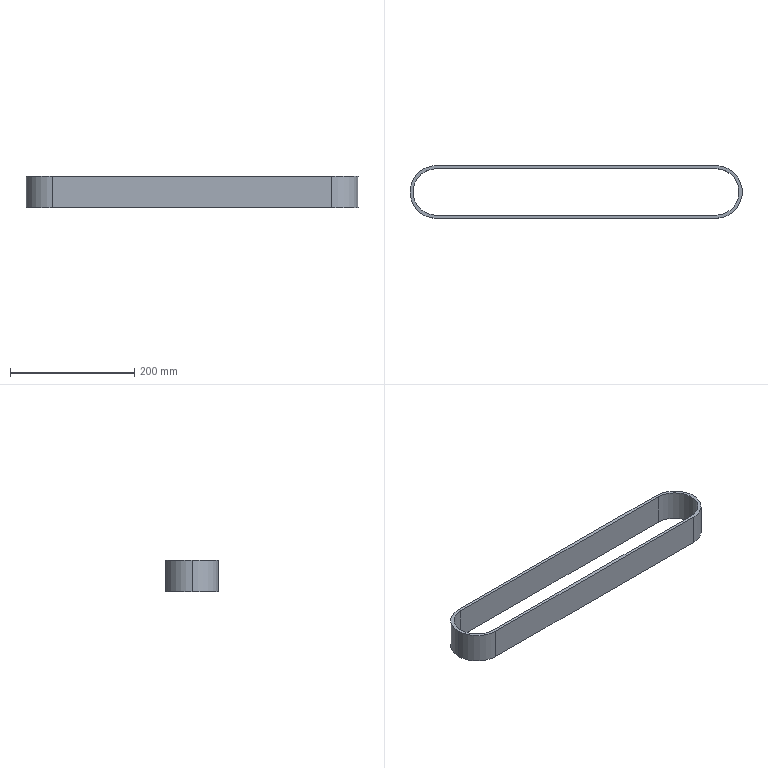Part | SolidWorks | features Extrusion 1 | 1 solid | 12 faces | box 535 x 85 x 50 mm | volume 287832 mm3 | cylinder 6 | plane 6 | commonest cylinder face diameters 75 x3 85 x3
STEP:
#1=CARTESIAN_POINT('',(-225.,37.5,50.));
#2=VERTEX_POINT('',#1);
#3=CARTESIAN_POINT('',(-262.5,0.,50.));
#4=VERTEX_POINT('',#3);
#5=CARTESIAN_POINT('',(-225.,0.,50.));
#6=DIRECTION('',(0.,0.,1.));
#7=DIRECTION('',(1.,0.,0.));
#8=AXIS2_PLACEMENT_3D('',#5,#6,#7);
#9=CIRCLE('',#8,37.5);
#10=EDGE_CURVE('',#2,#4,#9,.T.);
#11=ORIENTED_EDGE('',*,*,#10,.T.);
#12=CARTESIAN_POINT('',(-262.5,0.,0.));
#13=VERTEX_POINT('',#12);
#14=CARTESIAN_POINT('',(-262.5,0.,50.));
#15=DIRECTION('',(0.,0.,-1.));
#16=VECTOR('',#15,1000.);
#17=LINE('',#14,#16);
#18=EDGE_CURVE('',#4,#13,#17,.T.);
#19=ORIENTED_EDGE('',*,*,#18,.T.);
#20=CARTESIAN_POINT('',(-225.,37.5,0.));
#21=VERTEX_POINT('',#20);
#22=CARTESIAN_POINT('',(-225.,0.,0.));
#23=DIRECTION('',(0.,0.,1.));
#24=DIRECTION('',(1.,0.,0.));
#25=AXIS2_PLACEMENT_3D('',#22,#23,#24);
#26=CIRCLE('',#25,37.5);
#27=EDGE_CURVE('',#21,#13,#26,.T.);
#28=ORIENTED_EDGE('',*,*,#27,.F.);
#29=CARTESIAN_POINT('',(-225.,37.5,50.));
#30=DIRECTION('',(0.,0.,-1.));
#31=VECTOR('',#30,1000.);
#32=LINE('',#29,#31);
#33=EDGE_CURVE('',#2,#21,#32,.T.);
#34=ORIENTED_EDGE('',*,*,#33,.F.);
#35=EDGE_LOOP('',(#11,#19,#28,#34));
#36=FACE_OUTER_BOUND('',#35,.T.);
#37=CARTESIAN_POINT('',(-225.,0.,50.));
#38=DIRECTION('',(0.,0.,-1.));
#39=DIRECTION('',(-1.,0.,0.));
#40=AXIS2_PLACEMENT_3D('',#37,#38,#39);
#41=CYLINDRICAL_SURFACE('',#40,37.5);
#42=ADVANCED_FACE('',(#36),#41,.F.);
#43=CARTESIAN_POINT('',(-267.5,0.,50.));
#44=VERTEX_POINT('',#43);
#45=CARTESIAN_POINT('',(-225.,-42.5,50.));
#46=VERTEX_POINT('',#45);
#47=CARTESIAN_POINT('',(-225.,0.,50.));
#48=DIRECTION('',(0.,0.,1.));
#49=DIRECTION('',(1.,0.,0.));
#50=AXIS2_PLACEMENT_3D('',#47,#48,#49);
#51=CIRCLE('',#50,42.5);
#52=EDGE_CURVE('',#44,#46,#51,.T.);
#53=ORIENTED_EDGE('',*,*,#52,.F.);
#54=CARTESIAN_POINT('',(-267.5,0.,0.));
#55=VERTEX_POINT('',#54);
#56=CARTESIAN_POINT('',(-267.5,0.,50.));
#57=DIRECTION('',(0.,0.,-1.));
#58=VECTOR('',#57,1000.);
#59=LINE('',#56,#58);
#60=EDGE_CURVE('',#44,#55,#59,.T.);
#61=ORIENTED_EDGE('',*,*,#60,.T.);
#62=CARTESIAN_POINT('',(-225.,-42.5,0.));
#63=VERTEX_POINT('',#62);
#64=CARTESIAN_POINT('',(-225.,0.,0.));
#65=DIRECTION('',(0.,0.,1.));
#66=DIRECTION('',(1.,0.,0.));
#67=AXIS2_PLACEMENT_3D('',#64,#65,#66);
#68=CIRCLE('',#67,42.5);
#69=EDGE_CURVE('',#55,#63,#68,.T.);
#70=ORIENTED_EDGE('',*,*,#69,.T.);
#71=CARTESIAN_POINT('',(-225.,-42.5,50.));
#72=DIRECTION('',(0.,0.,-1.));
#73=VECTOR('',#72,1000.);
#74=LINE('',#71,#73);
#75=EDGE_CURVE('',#46,#63,#74,.T.);
#76=ORIENTED_EDGE('',*,*,#75,.F.);
#77=EDGE_LOOP('',(#53,#61,#70,#76));
#78=FACE_OUTER_BOUND('',#77,.T.);
#79=CARTESIAN_POINT('',(-225.,0.,50.));
#80=DIRECTION('',(0.,0.,-1.));
#81=DIRECTION('',(-1.,0.,0.));
#82=AXIS2_PLACEMENT_3D('',#79,#80,#81);
#83=CYLINDRICAL_SURFACE('',#82,42.5);
#84=ADVANCED_FACE('',(#78),#83,.T.);
#85=CARTESIAN_POINT('',(-225.,42.5,50.));
#86=VERTEX_POINT('',#85);
#87=CARTESIAN_POINT('',(-225.,0.,50.));
#88=DIRECTION('',(0.,0.,1.));
#89=DIRECTION('',(1.,0.,0.));
#90=AXIS2_PLACEMENT_3D('',#87,#88,#89);
#91=CIRCLE('',#90,42.5);
#92=EDGE_CURVE('',#86,#44,#91,.T.);
#93=ORIENTED_EDGE('',*,*,#92,.T.);
#94=ORIENTED_EDGE('',*,*,#52,.T.);
#95=CARTESIAN_POINT('',(225.,-42.5,50.));
#96=VERTEX_POINT('',#95);
#97=CARTESIAN_POINT('',(-225.,-42.5,50.));
#98=DIRECTION('',(1.,0.,0.));
#99=VECTOR('',#98,1000.);
#100=LINE('',#97,#99);
#101=EDGE_CURVE('',#46,#96,#100,.T.);
#102=ORIENTED_EDGE('',*,*,#101,.T.);
#103=CARTESIAN_POINT('',(225.,42.5,50.));
#104=VERTEX_POINT('',#103);
#105=CARTESIAN_POINT('',(225.,0.,50.));
#106=DIRECTION('',(0.,0.,1.));
#107=DIRECTION('',(1.,0.,0.));
#108=AXIS2_PLACEMENT_3D('',#105,#106,#107);
#109=CIRCLE('',#108,42.5);
#110=EDGE_CURVE('',#96,#104,#109,.T.);
#111=ORIENTED_EDGE('',*,*,#110,.T.);
#112=CARTESIAN_POINT('',(-225.,42.5,50.));
#113=DIRECTION('',(-1.,0.,0.));
#114=VECTOR('',#113,1000.);
#115=LINE('',#112,#114);
#116=EDGE_CURVE('',#104,#86,#115,.T.);
#117=ORIENTED_EDGE('',*,*,#116,.T.);
#118=EDGE_LOOP('',(#93,#94,#102,#111,#117));
#119=FACE_OUTER_BOUND('',#118,.T.);
#120=CARTESIAN_POINT('',(-225.,-37.5,50.));
#121=VERTEX_POINT('',#120);
#122=CARTESIAN_POINT('',(225.,-37.5,50.));
#123=VERTEX_POINT('',#122);
#124=CARTESIAN_POINT('',(-225.,-37.5,50.));
#125=DIRECTION('',(1.,0.,0.));
#126=VECTOR('',#125,1000.);
#127=LINE('',#124,#126);
#128=EDGE_CURVE('',#121,#123,#127,.T.);
#129=ORIENTED_EDGE('',*,*,#128,.F.);
#130=CARTESIAN_POINT('',(-225.,0.,50.));
#131=DIRECTION('',(0.,0.,1.));
#132=DIRECTION('',(1.,0.,0.));
#133=AXIS2_PLACEMENT_3D('',#130,#131,#132);
#134=CIRCLE('',#133,37.5);
#135=EDGE_CURVE('',#4,#121,#134,.T.);
#136=ORIENTED_EDGE('',*,*,#135,.F.);
#137=ORIENTED_EDGE('',*,*,#10,.F.);
#138=CARTESIAN_POINT('',(225.,37.5,50.));
#139=VERTEX_POINT('',#138);
#140=CARTESIAN_POINT('',(-225.,37.5,50.));
#141=DIRECTION('',(-1.,0.,0.));
#142=VECTOR('',#141,1000.);
#143=LINE('',#140,#142);
#144=EDGE_CURVE('',#139,#2,#143,.T.);
#145=ORIENTED_EDGE('',*,*,#144,.F.);
#146=CARTESIAN_POINT('',(225.,0.,50.));
#147=DIRECTION('',(0.,0.,1.));
#148=DIRECTION('',(1.,0.,0.));
#149=AXIS2_PLACEMENT_3D('',#146,#147,#148);
#150=CIRCLE('',#149,37.5);
#151=EDGE_CURVE('',#123,#139,#150,.T.);
#152=ORIENTED_EDGE('',*,*,#151,.F.);
#153=EDGE_LOOP('',(#129,#136,#137,#145,#152));
#154=FACE_BOUND('',#153,.T.);
#155=CARTESIAN_POINT('',(-225.,0.,50.));
#156=DIRECTION('',(0.,0.,1.));
#157=DIRECTION('',(1.,0.,0.));
#158=AXIS2_PLACEMENT_3D('',#155,#156,#157);
#159=PLANE('',#158);
#160=ADVANCED_FACE('',(#119,#154),#159,.T.);
#161=CARTESIAN_POINT('',(-225.,42.5,0.));
#162=VERTEX_POINT('',#161);
#163=CARTESIAN_POINT('',(-225.,0.,0.));
#164=DIRECTION('',(0.,0.,1.));
#165=DIRECTION('',(1.,0.,0.));
#166=AXIS2_PLACEMENT_3D('',#163,#164,#165);
#167=CIRCLE('',#166,42.5);
#168=EDGE_CURVE('',#162,#55,#167,.T.);
#169=ORIENTED_EDGE('',*,*,#168,.F.);
#170=CARTESIAN_POINT('',(225.,42.5,0.));
#171=VERTEX_POINT('',#170);
#172=CARTESIAN_POINT('',(-225.,42.5,0.));
#173=DIRECTION('',(-1.,0.,0.));
#174=VECTOR('',#173,1000.);
#175=LINE('',#172,#174);
#176=EDGE_CURVE('',#171,#162,#175,.T.);
#177=ORIENTED_EDGE('',*,*,#176,.F.);
#178=CARTESIAN_POINT('',(225.,-42.5,0.));
#179=VERTEX_POINT('',#178);
#180=CARTESIAN_POINT('',(225.,0.,0.));
#181=DIRECTION('',(0.,0.,1.));
#182=DIRECTION('',(1.,0.,0.));
#183=AXIS2_PLACEMENT_3D('',#180,#181,#182);
#184=CIRCLE('',#183,42.5);
#185=EDGE_CURVE('',#179,#171,#184,.T.);
#186=ORIENTED_EDGE('',*,*,#185,.F.);
#187=CARTESIAN_POINT('',(-225.,-42.5,0.));
#188=DIRECTION('',(1.,0.,0.));
#189=VECTOR('',#188,1000.);
#190=LINE('',#187,#189);
#191=EDGE_CURVE('',#63,#179,#190,.T.);
#192=ORIENTED_EDGE('',*,*,#191,.F.);
#193=ORIENTED_EDGE('',*,*,#69,.F.);
#194=EDGE_LOOP('',(#169,#177,#186,#192,#193));
#195=FACE_OUTER_BOUND('',#194,.T.);
#196=ORIENTED_EDGE('',*,*,#27,.T.);
#197=CARTESIAN_POINT('',(-225.,-37.5,0.));
#198=VERTEX_POINT('',#197);
#199=CARTESIAN_POINT('',(-225.,0.,0.));
#200=DIRECTION('',(0.,0.,1.));
#201=DIRECTION('',(1.,0.,0.));
#202=AXIS2_PLACEMENT_3D('',#199,#200,#201);
#203=CIRCLE('',#202,37.5);
#204=EDGE_CURVE('',#13,#198,#203,.T.);
#205=ORIENTED_EDGE('',*,*,#204,.T.);
#206=CARTESIAN_POINT('',(225.,-37.5,0.));
#207=VERTEX_POINT('',#206);
#208=CARTESIAN_POINT('',(-225.,-37.5,0.));
#209=DIRECTION('',(1.,0.,0.));
#210=VECTOR('',#209,1000.);
#211=LINE('',#208,#210);
#212=EDGE_CURVE('',#198,#207,#211,.T.);
#213=ORIENTED_EDGE('',*,*,#212,.T.);
#214=CARTESIAN_POINT('',(225.,37.5,0.));
#215=VERTEX_POINT('',#214);
#216=CARTESIAN_POINT('',(225.,0.,0.));
#217=DIRECTION('',(0.,0.,1.));
#218=DIRECTION('',(1.,0.,0.));
#219=AXIS2_PLACEMENT_3D('',#216,#217,#218);
#220=CIRCLE('',#219,37.5);
#221=EDGE_CURVE('',#207,#215,#220,.T.);
#222=ORIENTED_EDGE('',*,*,#221,.T.);
#223=CARTESIAN_POINT('',(-225.,37.5,0.));
#224=DIRECTION('',(-1.,0.,0.));
#225=VECTOR('',#224,1000.);
#226=LINE('',#223,#225);
#227=EDGE_CURVE('',#215,#21,#226,.T.);
#228=ORIENTED_EDGE('',*,*,#227,.T.);
#229=EDGE_LOOP('',(#196,#205,#213,#222,#228));
#230=FACE_BOUND('',#229,.T.);
#231=CARTESIAN_POINT('',(-225.,0.,0.));
#232=DIRECTION('',(0.,0.,1.));
#233=DIRECTION('',(1.,0.,0.));
#234=AXIS2_PLACEMENT_3D('',#231,#232,#233);
#235=PLANE('',#234);
#236=ADVANCED_FACE('',(#195,#230),#235,.F.);
#237=ORIENTED_EDGE('',*,*,#60,.F.);
#238=ORIENTED_EDGE('',*,*,#92,.F.);
#239=CARTESIAN_POINT('',(-225.,42.5,50.));
#240=DIRECTION('',(0.,0.,-1.));
#241=VECTOR('',#240,1000.);
#242=LINE('',#239,#241);
#243=EDGE_CURVE('',#86,#162,#242,.T.);
#244=ORIENTED_EDGE('',*,*,#243,.T.);
#245=ORIENTED_EDGE('',*,*,#168,.T.);
#246=EDGE_LOOP('',(#237,#238,#244,#245));
#247=FACE_OUTER_BOUND('',#246,.T.);
#248=CARTESIAN_POINT('',(-225.,0.,50.));
#249=DIRECTION('',(0.,0.,-1.));
#250=DIRECTION('',(-1.,0.,0.));
#251=AXIS2_PLACEMENT_3D('',#248,#249,#250);
#252=CYLINDRICAL_SURFACE('',#251,42.5);
#253=ADVANCED_FACE('',(#247),#252,.T.);
#254=ORIENTED_EDGE('',*,*,#191,.T.);
#255=CARTESIAN_POINT('',(225.,-42.5,50.));
#256=DIRECTION('',(0.,0.,-1.));
#257=VECTOR('',#256,1000.);
#258=LINE('',#255,#257);
#259=EDGE_CURVE('',#96,#179,#258,.T.);
#260=ORIENTED_EDGE('',*,*,#259,.F.);
#261=ORIENTED_EDGE('',*,*,#101,.F.);
#262=ORIENTED_EDGE('',*,*,#75,.T.);
#263=EDGE_LOOP('',(#254,#260,#261,#262));
#264=FACE_OUTER_BOUND('',#263,.T.);
#265=CARTESIAN_POINT('',(-225.,-42.5,50.));
#266=DIRECTION('',(0.,1.,0.));
#267=DIRECTION('',(-1.,0.,0.));
#268=AXIS2_PLACEMENT_3D('',#265,#266,#267);
#269=PLANE('',#268);
#270=ADVANCED_FACE('',(#264),#269,.F.);
#271=ORIENTED_EDGE('',*,*,#185,.T.);
#272=CARTESIAN_POINT('',(225.,42.5,50.));
#273=DIRECTION('',(0.,0.,-1.));
#274=VECTOR('',#273,1000.);
#275=LINE('',#272,#274);
#276=EDGE_CURVE('',#104,#171,#275,.T.);
#277=ORIENTED_EDGE('',*,*,#276,.F.);
#278=ORIENTED_EDGE('',*,*,#110,.F.);
#279=ORIENTED_EDGE('',*,*,#259,.T.);
#280=EDGE_LOOP('',(#271,#277,#278,#279));
#281=FACE_OUTER_BOUND('',#280,.T.);
#282=CARTESIAN_POINT('',(225.,0.,50.));
#283=DIRECTION('',(0.,0.,-1.));
#284=DIRECTION('',(-1.,0.,0.));
#285=AXIS2_PLACEMENT_3D('',#282,#283,#284);
#286=CYLINDRICAL_SURFACE('',#285,42.5);
#287=ADVANCED_FACE('',(#281),#286,.T.);
#288=ORIENTED_EDGE('',*,*,#176,.T.);
#289=ORIENTED_EDGE('',*,*,#243,.F.);
#290=ORIENTED_EDGE('',*,*,#116,.F.);
#291=ORIENTED_EDGE('',*,*,#276,.T.);
#292=EDGE_LOOP('',(#288,#289,#290,#291));
#293=FACE_OUTER_BOUND('',#292,.T.);
#294=CARTESIAN_POINT('',(-225.,42.5,50.));
#295=DIRECTION('',(0.,-1.,0.));
#296=DIRECTION('',(1.,0.,0.));
#297=AXIS2_PLACEMENT_3D('',#294,#295,#296);
#298=PLANE('',#297);
#299=ADVANCED_FACE('',(#293),#298,.F.);
#300=ORIENTED_EDGE('',*,*,#18,.F.);
#301=ORIENTED_EDGE('',*,*,#135,.T.);
#302=CARTESIAN_POINT('',(-225.,-37.5,50.));
#303=DIRECTION('',(0.,0.,-1.));
#304=VECTOR('',#303,1000.);
#305=LINE('',#302,#304);
#306=EDGE_CURVE('',#121,#198,#305,.T.);
#307=ORIENTED_EDGE('',*,*,#306,.T.);
#308=ORIENTED_EDGE('',*,*,#204,.F.);
#309=EDGE_LOOP('',(#300,#301,#307,#308));
#310=FACE_OUTER_BOUND('',#309,.T.);
#311=CARTESIAN_POINT('',(-225.,0.,50.));
#312=DIRECTION('',(0.,0.,-1.));
#313=DIRECTION('',(-1.,0.,0.));
#314=AXIS2_PLACEMENT_3D('',#311,#312,#313);
#315=CYLINDRICAL_SURFACE('',#314,37.5);
#316=ADVANCED_FACE('',(#310),#315,.F.);
#317=ORIENTED_EDGE('',*,*,#212,.F.);
#318=ORIENTED_EDGE('',*,*,#306,.F.);
#319=ORIENTED_EDGE('',*,*,#128,.T.);
#320=CARTESIAN_POINT('',(225.,-37.5,50.));
#321=DIRECTION('',(0.,0.,-1.));
#322=VECTOR('',#321,1000.);
#323=LINE('',#320,#322);
#324=EDGE_CURVE('',#123,#207,#323,.T.);
#325=ORIENTED_EDGE('',*,*,#324,.T.);
#326=EDGE_LOOP('',(#317,#318,#319,#325));
#327=FACE_OUTER_BOUND('',#326,.T.);
#328=CARTESIAN_POINT('',(-225.,-37.5,50.));
#329=DIRECTION('',(0.,1.,0.));
#330=DIRECTION('',(0.,0.,1.));
#331=AXIS2_PLACEMENT_3D('',#328,#329,#330);
#332=PLANE('',#331);
#333=ADVANCED_FACE('',(#327),#332,.T.);
#334=ORIENTED_EDGE('',*,*,#221,.F.);
#335=ORIENTED_EDGE('',*,*,#324,.F.);
#336=ORIENTED_EDGE('',*,*,#151,.T.);
#337=CARTESIAN_POINT('',(225.,37.5,50.));
#338=DIRECTION('',(0.,0.,-1.));
#339=VECTOR('',#338,1000.);
#340=LINE('',#337,#339);
#341=EDGE_CURVE('',#139,#215,#340,.T.);
#342=ORIENTED_EDGE('',*,*,#341,.T.);
#343=EDGE_LOOP('',(#334,#335,#336,#342));
#344=FACE_OUTER_BOUND('',#343,.T.);
#345=CARTESIAN_POINT('',(225.,0.,50.));
#346=DIRECTION('',(0.,0.,-1.));
#347=DIRECTION('',(-1.,0.,0.));
#348=AXIS2_PLACEMENT_3D('',#345,#346,#347);
#349=CYLINDRICAL_SURFACE('',#348,37.5);
#350=ADVANCED_FACE('',(#344),#349,.F.);
#351=ORIENTED_EDGE('',*,*,#227,.F.);
#352=ORIENTED_EDGE('',*,*,#341,.F.);
#353=ORIENTED_EDGE('',*,*,#144,.T.);
#354=ORIENTED_EDGE('',*,*,#33,.T.);
#355=EDGE_LOOP('',(#351,#352,#353,#354));
#356=FACE_OUTER_BOUND('',#355,.T.);
#357=CARTESIAN_POINT('',(-225.,37.5,50.));
#358=DIRECTION('',(0.,-1.,0.));
#359=DIRECTION('',(0.,0.,-1.));
#360=AXIS2_PLACEMENT_3D('',#357,#358,#359);
#361=PLANE('',#360);
#362=ADVANCED_FACE('',(#356),#361,.T.);
#363=CLOSED_SHELL('',(#42,#84,#160,#236,#253,#270,#287,#299,#316,#333,#350,#362));
#364=MANIFOLD_SOLID_BREP('',#363);
#365=CARTESIAN_POINT('',(0.,0.,0.));
#366=DIRECTION('',(0.,0.,1.));
#367=DIRECTION('',(1.,0.,0.));
#368=AXIS2_PLACEMENT_3D('',#365,#366,#367);
#369=(LENGTH_UNIT()NAMED_UNIT(*)SI_UNIT(.MILLI.,.METRE.));
#370=UNCERTAINTY_MEASURE_WITH_UNIT(LENGTH_MEASURE(0.00001),#369,'','');
#371=(NAMED_UNIT(*)PLANE_ANGLE_UNIT()SI_UNIT($,.RADIAN.));
#372=(NAMED_UNIT(*)SI_UNIT($,.STERADIAN.)SOLID_ANGLE_UNIT());
#373=(GEOMETRIC_REPRESENTATION_CONTEXT(3)GLOBAL_UNCERTAINTY_ASSIGNED_CONTEXT((#370))GLOBAL_UNIT_ASSIGNED_CONTEXT((#369,#371,#372))REPRESENTATION_CONTEXT('',''));
#374=ADVANCED_BREP_SHAPE_REPRESENTATION('',(#364,#368),#373);